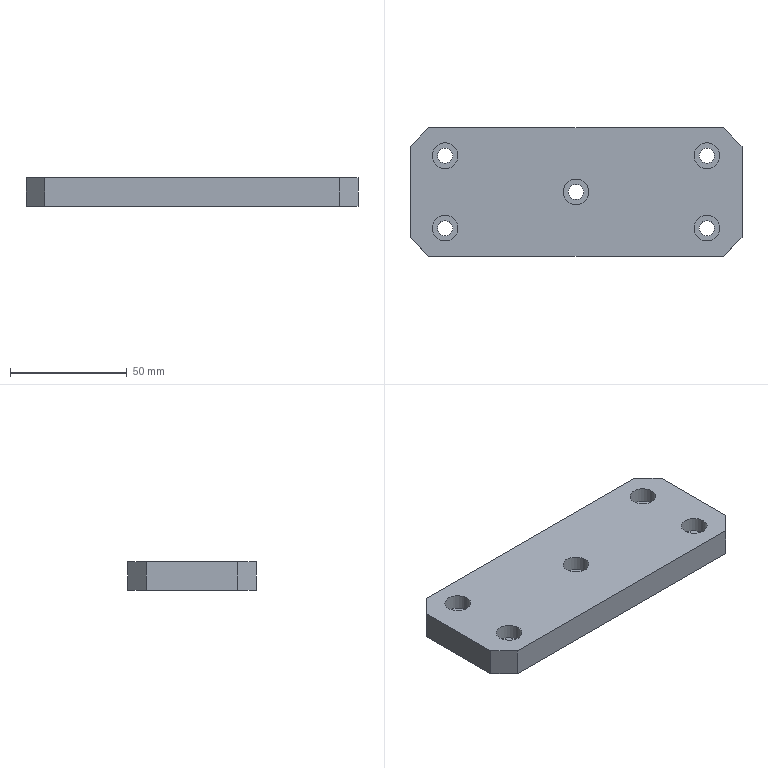Part | STEP file | P011002S004-006 | 1 solid | 25 faces | box 142 x 55 x 12 mm | volume 88183 mm3 | plane 15 | cylinder 10 | commonest cylinder face diameters 6.5 x5 11 x5